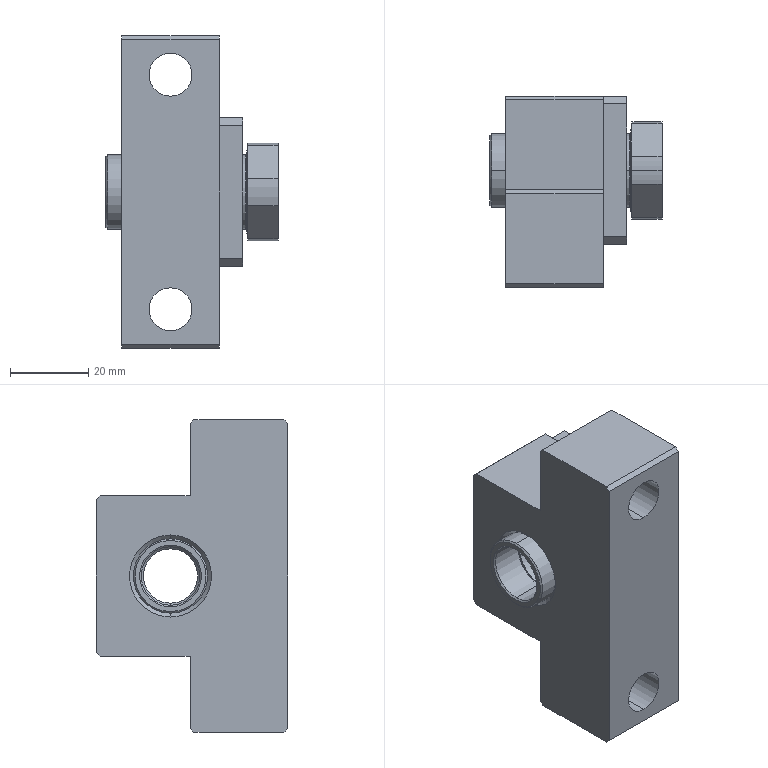Part | SolidWorks | features AEMSimFeature 1 | 9 solids | 286 faces | box 44 x 49 x 80 mm | volume 74061 mm3 | plane 141 | cylinder 89 | cone 56 | commonest cylinder face diameters 2.459 x10 3 x8 3.5 x8 5.5 x8 7 x8 19 x8